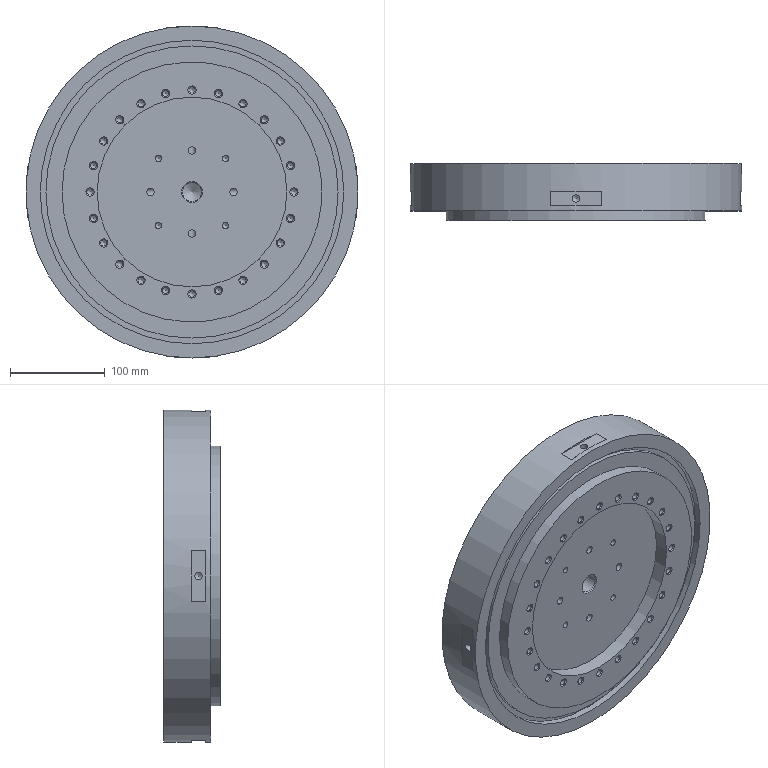Part | STEP file | Upper part | 1 solid | 172 faces | box 350 x 60 x 350 mm | volume 4244226 mm3 | cone 76 | cylinder 74 | plane 22 | commonest cylinder face diameters 6.647 x28 4.917 x20 8 x16 78 x4 20 x1 200 x1